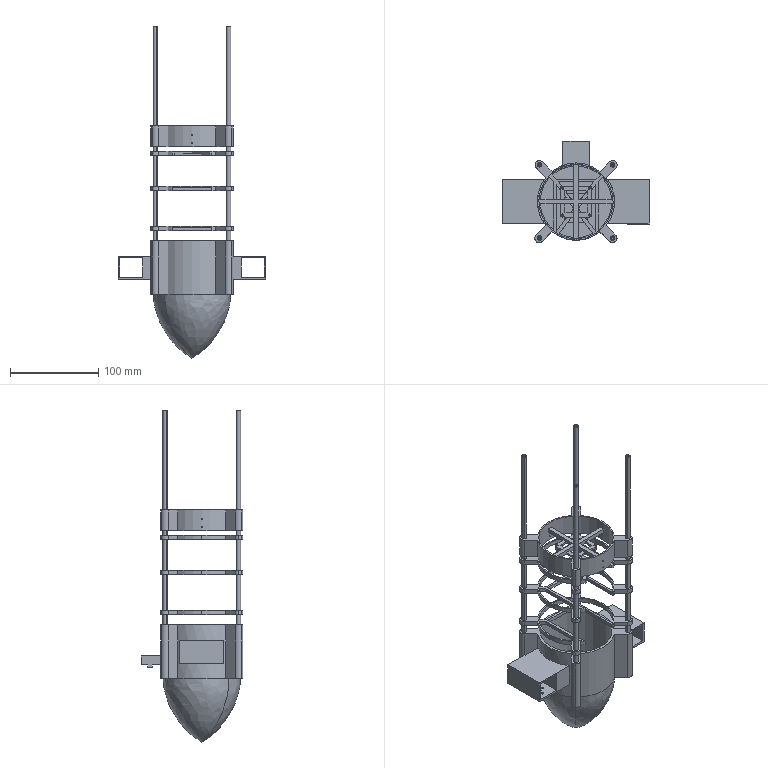Part | SolidWorks | features ReferencePattern 3, CompositeCurve 1, LocalCirPattern 1 | 10 solids | 400 faces | box 167.293 x 115.141 x 375.279 mm | volume 493659 mm3 | cylinder 210 | plane 184 | cone 4 | spline 2 | commonest cylinder face diameters 5 x56 10 x46 87.2 x26 1 x24 3 x16 84.2 x16